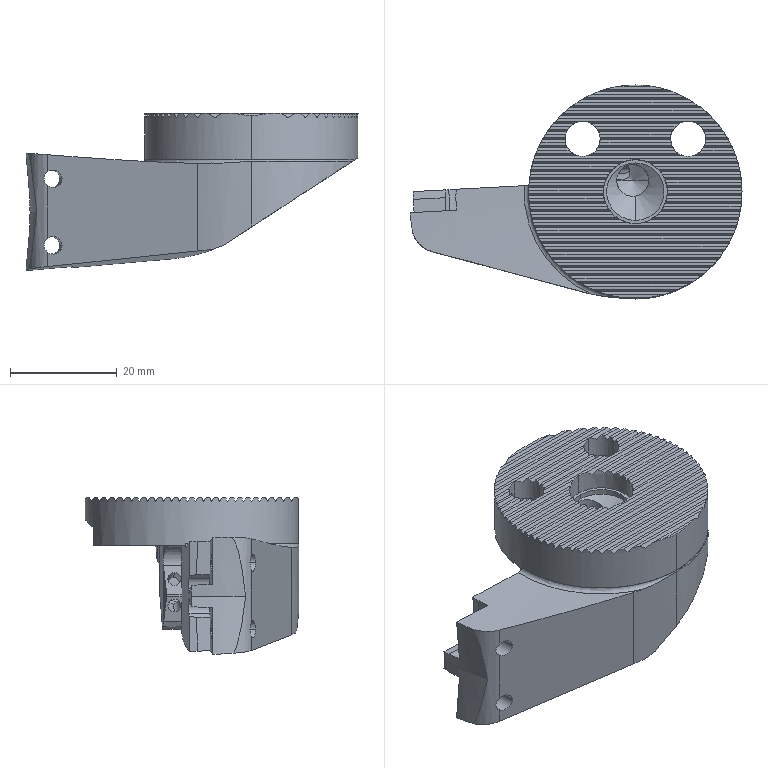Part | 1 solid | 201 faces | volume 23613 mm3 | plane 158 | cylinder 33 | cone 8 | torus 1 | spline 1 | commonest cylinder face diameters 11 x5 2.5 x4 3.3 x4 6.6 x4 6 x3 3.5 x2